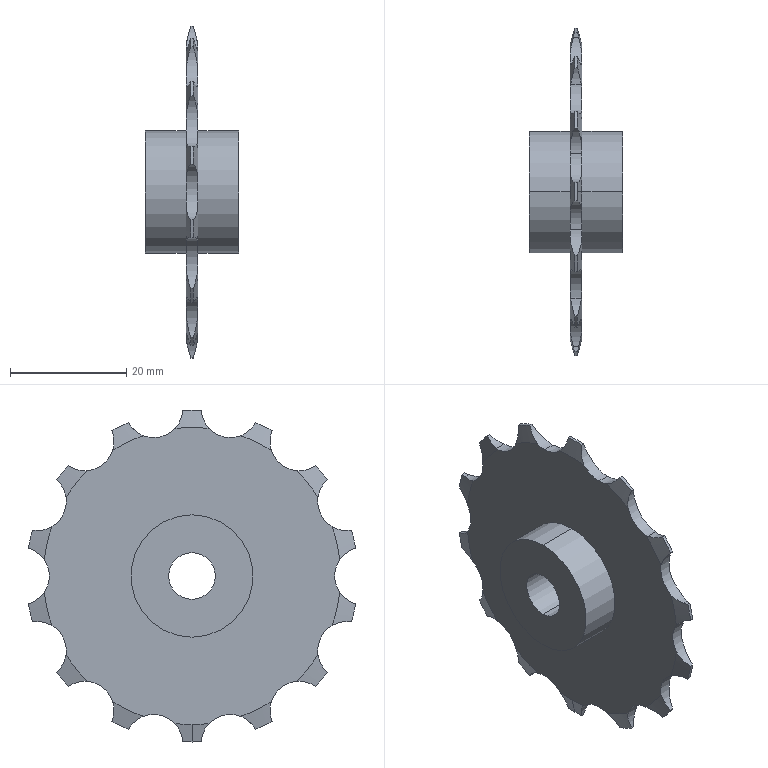Part | STEP file | Metal teeth for metal toothed Idler | 1 solid | 75 faces | box 16 x 56.186 x 57 mm | volume 8251 mm3 | cylinder 41 | cone 30 | plane 4 | commonest cylinder face diameters 10 x20 57 x15 21 x4 8 x2